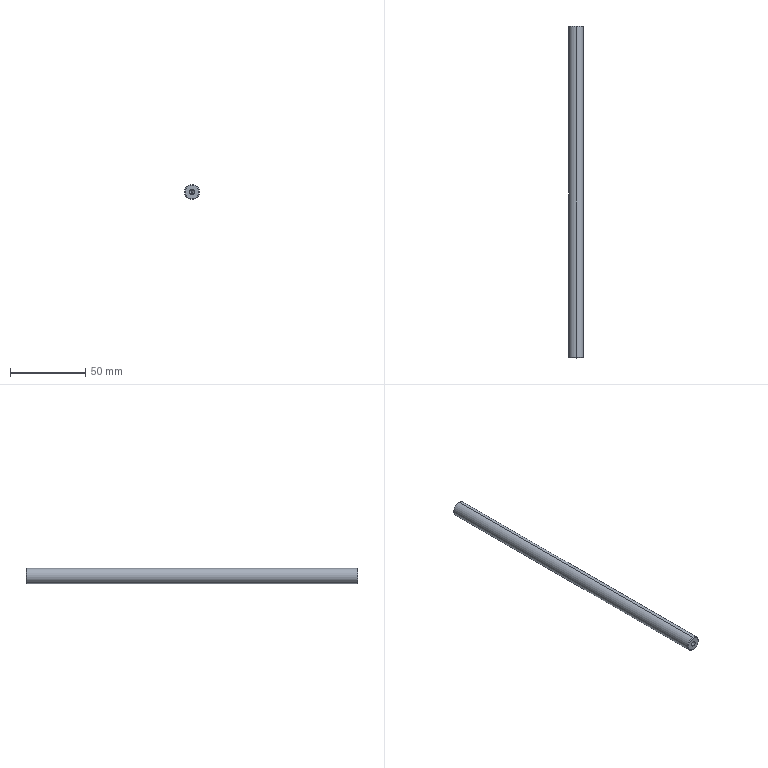Part | SolidWorks | features HoleWzd 2, Chamfer 1, Extrusion 1 | 1 solid | 16 faces | box 10 x 220 x 10 mm | volume 17093 mm3 | cone 8 | cylinder 6 | plane 2 | commonest cylinder face diameters 3.3 x4 10 x2
STEP:
#1=CARTESIAN_POINT('',(0.,-99.9,1.65));
#2=VERTEX_POINT('',#1);
#3=CARTESIAN_POINT('',(0.,-99.9,-1.65));
#4=VERTEX_POINT('',#3);
#5=CARTESIAN_POINT('',(0.,-99.9,0.));
#6=DIRECTION('',(0.,-1.,0.));
#7=DIRECTION('',(0.,0.,-1.));
#8=AXIS2_PLACEMENT_3D('',#5,#6,#7);
#9=CIRCLE('',#8,1.65);
#10=EDGE_CURVE('',#2,#4,#9,.T.);
#11=ORIENTED_EDGE('',*,*,#10,.F.);
#12=CARTESIAN_POINT('',(0.,-110.,1.65));
#13=VERTEX_POINT('',#12);
#14=CARTESIAN_POINT('',(0.,-110.,1.65));
#15=DIRECTION('',(0.,-1.,0.));
#16=VECTOR('',#15,1000.);
#17=LINE('',#14,#16);
#18=EDGE_CURVE('',#2,#13,#17,.T.);
#19=ORIENTED_EDGE('',*,*,#18,.T.);
#20=CARTESIAN_POINT('',(0.,-110.,-1.65));
#21=VERTEX_POINT('',#20);
#22=CARTESIAN_POINT('',(0.,-110.,0.));
#23=DIRECTION('',(0.,-1.,0.));
#24=DIRECTION('',(0.,0.,-1.));
#25=AXIS2_PLACEMENT_3D('',#22,#23,#24);
#26=CIRCLE('',#25,1.65);
#27=EDGE_CURVE('',#13,#21,#26,.T.);
#28=ORIENTED_EDGE('',*,*,#27,.T.);
#29=CARTESIAN_POINT('',(0.,-110.,-1.65));
#30=DIRECTION('',(0.,-1.,0.));
#31=VECTOR('',#30,1000.);
#32=LINE('',#29,#31);
#33=EDGE_CURVE('',#4,#21,#32,.T.);
#34=ORIENTED_EDGE('',*,*,#33,.F.);
#35=EDGE_LOOP('',(#11,#19,#28,#34));
#36=FACE_OUTER_BOUND('',#35,.T.);
#37=CARTESIAN_POINT('',(0.,-110.,0.));
#38=DIRECTION('',(0.,-1.,0.));
#39=DIRECTION('',(0.,0.,-1.));
#40=AXIS2_PLACEMENT_3D('',#37,#38,#39);
#41=CYLINDRICAL_SURFACE('',#40,1.65);
#42=ADVANCED_FACE('',(#36),#41,.F.);
#43=CARTESIAN_POINT('',(0.,-98.909,0.));
#44=VERTEX_POINT('',#43);
#45=CARTESIAN_POINT('',(0.,-99.9,-1.65));
#46=DIRECTION('',(0.,-0.515,-0.8572));
#47=VECTOR('',#46,1000.);
#48=LINE('',#45,#47);
#49=EDGE_CURVE('',#44,#4,#48,.T.);
#50=ORIENTED_EDGE('',*,*,#49,.F.);
#51=CARTESIAN_POINT('',(0.,-99.9,1.65));
#52=DIRECTION('',(0.,-0.515,0.8572));
#53=VECTOR('',#52,1000.);
#54=LINE('',#51,#53);
#55=EDGE_CURVE('',#44,#2,#54,.T.);
#56=ORIENTED_EDGE('',*,*,#55,.T.);
#57=ORIENTED_EDGE('',*,*,#10,.T.);
#58=EDGE_LOOP('',(#50,#56,#57));
#59=FACE_OUTER_BOUND('',#58,.T.);
#60=CARTESIAN_POINT('',(0.,-99.9,0.));
#61=DIRECTION('',(0.,-1.,0.));
#62=DIRECTION('',(0.,0.,-1.));
#63=AXIS2_PLACEMENT_3D('',#60,#61,#62);
#64=CONICAL_SURFACE('',#63,1.65,1.03);
#65=ADVANCED_FACE('',(#59),#64,.F.);
#66=CARTESIAN_POINT('',(0.,99.9,-1.65));
#67=VERTEX_POINT('',#66);
#68=CARTESIAN_POINT('',(0.,99.9,1.65));
#69=VERTEX_POINT('',#68);
#70=CARTESIAN_POINT('',(0.,99.9,0.));
#71=DIRECTION('',(0.,1.,0.));
#72=DIRECTION('',(0.,0.,1.));
#73=AXIS2_PLACEMENT_3D('',#70,#71,#72);
#74=CIRCLE('',#73,1.65);
#75=EDGE_CURVE('',#67,#69,#74,.T.);
#76=ORIENTED_EDGE('',*,*,#75,.F.);
#77=CARTESIAN_POINT('',(0.,110.,-1.65));
#78=VERTEX_POINT('',#77);
#79=CARTESIAN_POINT('',(0.,110.,-1.65));
#80=DIRECTION('',(0.,1.,0.));
#81=VECTOR('',#80,1000.);
#82=LINE('',#79,#81);
#83=EDGE_CURVE('',#67,#78,#82,.T.);
#84=ORIENTED_EDGE('',*,*,#83,.T.);
#85=CARTESIAN_POINT('',(0.,110.,1.65));
#86=VERTEX_POINT('',#85);
#87=CARTESIAN_POINT('',(0.,110.,0.));
#88=DIRECTION('',(0.,1.,0.));
#89=DIRECTION('',(0.,0.,1.));
#90=AXIS2_PLACEMENT_3D('',#87,#88,#89);
#91=CIRCLE('',#90,1.65);
#92=EDGE_CURVE('',#78,#86,#91,.T.);
#93=ORIENTED_EDGE('',*,*,#92,.T.);
#94=CARTESIAN_POINT('',(0.,110.,1.65));
#95=DIRECTION('',(0.,1.,0.));
#96=VECTOR('',#95,1000.);
#97=LINE('',#94,#96);
#98=EDGE_CURVE('',#69,#86,#97,.T.);
#99=ORIENTED_EDGE('',*,*,#98,.F.);
#100=EDGE_LOOP('',(#76,#84,#93,#99));
#101=FACE_OUTER_BOUND('',#100,.T.);
#102=CARTESIAN_POINT('',(0.,110.,0.));
#103=DIRECTION('',(0.,1.,0.));
#104=DIRECTION('',(0.,0.,1.));
#105=AXIS2_PLACEMENT_3D('',#102,#103,#104);
#106=CYLINDRICAL_SURFACE('',#105,1.65);
#107=ADVANCED_FACE('',(#101),#106,.F.);
#108=CARTESIAN_POINT('',(0.,98.909,0.));
#109=VERTEX_POINT('',#108);
#110=CARTESIAN_POINT('',(0.,99.9,1.65));
#111=DIRECTION('',(0.,0.515,0.8572));
#112=VECTOR('',#111,1000.);
#113=LINE('',#110,#112);
#114=EDGE_CURVE('',#109,#69,#113,.T.);
#115=ORIENTED_EDGE('',*,*,#114,.F.);
#116=CARTESIAN_POINT('',(0.,99.9,-1.65));
#117=DIRECTION('',(0.,0.515,-0.8572));
#118=VECTOR('',#117,1000.);
#119=LINE('',#116,#118);
#120=EDGE_CURVE('',#109,#67,#119,.T.);
#121=ORIENTED_EDGE('',*,*,#120,.T.);
#122=ORIENTED_EDGE('',*,*,#75,.T.);
#123=EDGE_LOOP('',(#115,#121,#122));
#124=FACE_OUTER_BOUND('',#123,.T.);
#125=CARTESIAN_POINT('',(0.,99.9,0.));
#126=DIRECTION('',(0.,1.,0.));
#127=DIRECTION('',(0.,0.,1.));
#128=AXIS2_PLACEMENT_3D('',#125,#126,#127);
#129=CONICAL_SURFACE('',#128,1.65,1.03);
#130=ADVANCED_FACE('',(#124),#129,.F.);
#131=CARTESIAN_POINT('',(0.,110.,4.5));
#132=VERTEX_POINT('',#131);
#133=CARTESIAN_POINT('',(0.,110.,-4.5));
#134=VERTEX_POINT('',#133);
#135=CARTESIAN_POINT('',(0.,110.,0.));
#136=DIRECTION('',(0.,1.,0.));
#137=DIRECTION('',(0.,0.,1.));
#138=AXIS2_PLACEMENT_3D('',#135,#136,#137);
#139=CIRCLE('',#138,4.5);
#140=EDGE_CURVE('',#132,#134,#139,.T.);
#141=ORIENTED_EDGE('',*,*,#140,.F.);
#142=CARTESIAN_POINT('',(0.,109.5,5.));
#143=VERTEX_POINT('',#142);
#144=CARTESIAN_POINT('',(0.,110.,4.5));
#145=DIRECTION('',(0.,-0.7071,0.7071));
#146=VECTOR('',#145,1000.);
#147=LINE('',#144,#146);
#148=EDGE_CURVE('',#132,#143,#147,.T.);
#149=ORIENTED_EDGE('',*,*,#148,.T.);
#150=CARTESIAN_POINT('',(0.,109.5,-5.));
#151=VERTEX_POINT('',#150);
#152=CARTESIAN_POINT('',(0.,109.5,0.));
#153=DIRECTION('',(0.,-1.,0.));
#154=DIRECTION('',(0.,0.,1.));
#155=AXIS2_PLACEMENT_3D('',#152,#153,#154);
#156=CIRCLE('',#155,5.);
#157=EDGE_CURVE('',#151,#143,#156,.T.);
#158=ORIENTED_EDGE('',*,*,#157,.F.);
#159=CARTESIAN_POINT('',(0.,110.,-4.5));
#160=DIRECTION('',(0.,-0.7071,-0.7071));
#161=VECTOR('',#160,1000.);
#162=LINE('',#159,#161);
#163=EDGE_CURVE('',#134,#151,#162,.T.);
#164=ORIENTED_EDGE('',*,*,#163,.F.);
#165=EDGE_LOOP('',(#141,#149,#158,#164));
#166=FACE_OUTER_BOUND('',#165,.T.);
#167=CARTESIAN_POINT('',(0.,110.,0.));
#168=DIRECTION('',(0.,-1.,0.));
#169=DIRECTION('',(0.,0.,-1.));
#170=AXIS2_PLACEMENT_3D('',#167,#168,#169);
#171=CONICAL_SURFACE('',#170,4.5,0.7854);
#172=ADVANCED_FACE('',(#166),#171,.T.);
#173=CARTESIAN_POINT('',(0.,-110.,-4.5));
#174=VERTEX_POINT('',#173);
#175=CARTESIAN_POINT('',(0.,-110.,4.5));
#176=VERTEX_POINT('',#175);
#177=CARTESIAN_POINT('',(0.,-110.,0.));
#178=DIRECTION('',(0.,-1.,0.));
#179=DIRECTION('',(0.,0.,1.));
#180=AXIS2_PLACEMENT_3D('',#177,#178,#179);
#181=CIRCLE('',#180,4.5);
#182=EDGE_CURVE('',#174,#176,#181,.T.);
#183=ORIENTED_EDGE('',*,*,#182,.F.);
#184=CARTESIAN_POINT('',(0.,-109.5,-5.));
#185=VERTEX_POINT('',#184);
#186=CARTESIAN_POINT('',(0.,-109.5,-5.));
#187=DIRECTION('',(0.,0.7071,-0.7071));
#188=VECTOR('',#187,1000.);
#189=LINE('',#186,#188);
#190=EDGE_CURVE('',#174,#185,#189,.T.);
#191=ORIENTED_EDGE('',*,*,#190,.T.);
#192=CARTESIAN_POINT('',(0.,-109.5,5.));
#193=VERTEX_POINT('',#192);
#194=CARTESIAN_POINT('',(0.,-109.5,0.));
#195=DIRECTION('',(0.,1.,0.));
#196=DIRECTION('',(0.,0.,1.));
#197=AXIS2_PLACEMENT_3D('',#194,#195,#196);
#198=CIRCLE('',#197,5.);
#199=EDGE_CURVE('',#193,#185,#198,.T.);
#200=ORIENTED_EDGE('',*,*,#199,.F.);
#201=CARTESIAN_POINT('',(0.,-109.5,5.));
#202=DIRECTION('',(0.,0.7071,0.7071));
#203=VECTOR('',#202,1000.);
#204=LINE('',#201,#203);
#205=EDGE_CURVE('',#176,#193,#204,.T.);
#206=ORIENTED_EDGE('',*,*,#205,.F.);
#207=EDGE_LOOP('',(#183,#191,#200,#206));
#208=FACE_OUTER_BOUND('',#207,.T.);
#209=CARTESIAN_POINT('',(0.,-109.5,0.));
#210=DIRECTION('',(0.,1.,0.));
#211=DIRECTION('',(0.,0.,1.));
#212=AXIS2_PLACEMENT_3D('',#209,#210,#211);
#213=CONICAL_SURFACE('',#212,5.,0.7854);
#214=ADVANCED_FACE('',(#208),#213,.T.);
#215=ORIENTED_EDGE('',*,*,#157,.T.);
#216=CARTESIAN_POINT('',(0.,110.,5.));
#217=DIRECTION('',(0.,-1.,0.));
#218=VECTOR('',#217,1000.);
#219=LINE('',#216,#218);
#220=EDGE_CURVE('',#143,#193,#219,.T.);
#221=ORIENTED_EDGE('',*,*,#220,.T.);
#222=ORIENTED_EDGE('',*,*,#199,.T.);
#223=CARTESIAN_POINT('',(0.,110.,-5.));
#224=DIRECTION('',(0.,-1.,0.));
#225=VECTOR('',#224,1000.);
#226=LINE('',#223,#225);
#227=EDGE_CURVE('',#151,#185,#226,.T.);
#228=ORIENTED_EDGE('',*,*,#227,.F.);
#229=EDGE_LOOP('',(#215,#221,#222,#228));
#230=FACE_OUTER_BOUND('',#229,.T.);
#231=CARTESIAN_POINT('',(0.,110.,0.));
#232=DIRECTION('',(0.,-1.,0.));
#233=DIRECTION('',(0.,0.,-1.));
#234=AXIS2_PLACEMENT_3D('',#231,#232,#233);
#235=CYLINDRICAL_SURFACE('',#234,5.);
#236=ADVANCED_FACE('',(#230),#235,.T.);
#237=ORIENTED_EDGE('',*,*,#220,.F.);
#238=CARTESIAN_POINT('',(0.,109.5,0.));
#239=DIRECTION('',(0.,-1.,0.));
#240=DIRECTION('',(0.,0.,1.));
#241=AXIS2_PLACEMENT_3D('',#238,#239,#240);
#242=CIRCLE('',#241,5.);
#243=EDGE_CURVE('',#143,#151,#242,.T.);
#244=ORIENTED_EDGE('',*,*,#243,.T.);
#245=ORIENTED_EDGE('',*,*,#227,.T.);
#246=CARTESIAN_POINT('',(0.,-109.5,0.));
#247=DIRECTION('',(0.,1.,0.));
#248=DIRECTION('',(0.,0.,1.));
#249=AXIS2_PLACEMENT_3D('',#246,#247,#248);
#250=CIRCLE('',#249,5.);
#251=EDGE_CURVE('',#185,#193,#250,.T.);
#252=ORIENTED_EDGE('',*,*,#251,.T.);
#253=EDGE_LOOP('',(#237,#244,#245,#252));
#254=FACE_OUTER_BOUND('',#253,.T.);
#255=CARTESIAN_POINT('',(0.,110.,0.));
#256=DIRECTION('',(0.,-1.,0.));
#257=DIRECTION('',(0.,0.,-1.));
#258=AXIS2_PLACEMENT_3D('',#255,#256,#257);
#259=CYLINDRICAL_SURFACE('',#258,5.);
#260=ADVANCED_FACE('',(#254),#259,.T.);
#261=CARTESIAN_POINT('',(0.,110.,0.));
#262=DIRECTION('',(0.,1.,0.));
#263=DIRECTION('',(0.,0.,1.));
#264=AXIS2_PLACEMENT_3D('',#261,#262,#263);
#265=CIRCLE('',#264,1.65);
#266=EDGE_CURVE('',#86,#78,#265,.T.);
#267=ORIENTED_EDGE('',*,*,#266,.F.);
#268=ORIENTED_EDGE('',*,*,#92,.F.);
#269=EDGE_LOOP('',(#267,#268));
#270=FACE_BOUND('',#269,.T.);
#271=CARTESIAN_POINT('',(0.,110.,0.));
#272=DIRECTION('',(0.,1.,0.));
#273=DIRECTION('',(0.,0.,1.));
#274=AXIS2_PLACEMENT_3D('',#271,#272,#273);
#275=CIRCLE('',#274,4.5);
#276=EDGE_CURVE('',#134,#132,#275,.T.);
#277=ORIENTED_EDGE('',*,*,#276,.T.);
#278=ORIENTED_EDGE('',*,*,#140,.T.);
#279=EDGE_LOOP('',(#277,#278));
#280=FACE_OUTER_BOUND('',#279,.T.);
#281=CARTESIAN_POINT('',(0.,110.,0.));
#282=DIRECTION('',(0.,1.,0.));
#283=DIRECTION('',(0.,0.,1.));
#284=AXIS2_PLACEMENT_3D('',#281,#282,#283);
#285=PLANE('',#284);
#286=ADVANCED_FACE('',(#270,#280),#285,.T.);
#287=CARTESIAN_POINT('',(0.,-110.,0.));
#288=DIRECTION('',(0.,-1.,0.));
#289=DIRECTION('',(0.,0.,-1.));
#290=AXIS2_PLACEMENT_3D('',#287,#288,#289);
#291=CIRCLE('',#290,1.65);
#292=EDGE_CURVE('',#21,#13,#291,.T.);
#293=ORIENTED_EDGE('',*,*,#292,.F.);
#294=ORIENTED_EDGE('',*,*,#27,.F.);
#295=EDGE_LOOP('',(#293,#294));
#296=FACE_BOUND('',#295,.T.);
#297=CARTESIAN_POINT('',(0.,-110.,0.));
#298=DIRECTION('',(0.,-1.,0.));
#299=DIRECTION('',(0.,0.,1.));
#300=AXIS2_PLACEMENT_3D('',#297,#298,#299);
#301=CIRCLE('',#300,4.5);
#302=EDGE_CURVE('',#176,#174,#301,.T.);
#303=ORIENTED_EDGE('',*,*,#302,.T.);
#304=ORIENTED_EDGE('',*,*,#182,.T.);
#305=EDGE_LOOP('',(#303,#304));
#306=FACE_OUTER_BOUND('',#305,.T.);
#307=CARTESIAN_POINT('',(0.,-110.,0.));
#308=DIRECTION('',(0.,1.,0.));
#309=DIRECTION('',(0.,0.,1.));
#310=AXIS2_PLACEMENT_3D('',#307,#308,#309);
#311=PLANE('',#310);
#312=ADVANCED_FACE('',(#296,#306),#311,.F.);
#313=ORIENTED_EDGE('',*,*,#190,.F.);
#314=ORIENTED_EDGE('',*,*,#302,.F.);
#315=ORIENTED_EDGE('',*,*,#205,.T.);
#316=ORIENTED_EDGE('',*,*,#251,.F.);
#317=EDGE_LOOP('',(#313,#314,#315,#316));
#318=FACE_OUTER_BOUND('',#317,.T.);
#319=CARTESIAN_POINT('',(0.,-109.5,0.));
#320=DIRECTION('',(0.,1.,0.));
#321=DIRECTION('',(0.,0.,1.));
#322=AXIS2_PLACEMENT_3D('',#319,#320,#321);
#323=CONICAL_SURFACE('',#322,5.,0.7854);
#324=ADVANCED_FACE('',(#318),#323,.T.);
#325=ORIENTED_EDGE('',*,*,#148,.F.);
#326=ORIENTED_EDGE('',*,*,#276,.F.);
#327=ORIENTED_EDGE('',*,*,#163,.T.);
#328=ORIENTED_EDGE('',*,*,#243,.F.);
#329=EDGE_LOOP('',(#325,#326,#327,#328));
#330=FACE_OUTER_BOUND('',#329,.T.);
#331=CARTESIAN_POINT('',(0.,110.,0.));
#332=DIRECTION('',(0.,-1.,0.));
#333=DIRECTION('',(0.,0.,-1.));
#334=AXIS2_PLACEMENT_3D('',#331,#332,#333);
#335=CONICAL_SURFACE('',#334,4.5,0.7854);
#336=ADVANCED_FACE('',(#330),#335,.T.);
#337=ORIENTED_EDGE('',*,*,#120,.F.);
#338=ORIENTED_EDGE('',*,*,#114,.T.);
#339=CARTESIAN_POINT('',(0.,99.9,0.));
#340=DIRECTION('',(0.,1.,0.));
#341=DIRECTION('',(0.,0.,1.));
#342=AXIS2_PLACEMENT_3D('',#339,#340,#341);
#343=CIRCLE('',#342,1.65);
#344=EDGE_CURVE('',#69,#67,#343,.T.);
#345=ORIENTED_EDGE('',*,*,#344,.T.);
#346=EDGE_LOOP('',(#337,#338,#345));
#347=FACE_OUTER_BOUND('',#346,.T.);
#348=CARTESIAN_POINT('',(0.,99.9,0.));
#349=DIRECTION('',(0.,1.,0.));
#350=DIRECTION('',(0.,0.,1.));
#351=AXIS2_PLACEMENT_3D('',#348,#349,#350);
#352=CONICAL_SURFACE('',#351,1.65,1.03);
#353=ADVANCED_FACE('',(#347),#352,.F.);
#354=ORIENTED_EDGE('',*,*,#83,.F.);
#355=ORIENTED_EDGE('',*,*,#344,.F.);
#356=ORIENTED_EDGE('',*,*,#98,.T.);
#357=ORIENTED_EDGE('',*,*,#266,.T.);
#358=EDGE_LOOP('',(#354,#355,#356,#357));
#359=FACE_OUTER_BOUND('',#358,.T.);
#360=CARTESIAN_POINT('',(0.,110.,0.));
#361=DIRECTION('',(0.,1.,0.));
#362=DIRECTION('',(0.,0.,1.));
#363=AXIS2_PLACEMENT_3D('',#360,#361,#362);
#364=CYLINDRICAL_SURFACE('',#363,1.65);
#365=ADVANCED_FACE('',(#359),#364,.F.);
#366=ORIENTED_EDGE('',*,*,#55,.F.);
#367=ORIENTED_EDGE('',*,*,#49,.T.);
#368=CARTESIAN_POINT('',(0.,-99.9,0.));
#369=DIRECTION('',(0.,-1.,0.));
#370=DIRECTION('',(0.,0.,-1.));
#371=AXIS2_PLACEMENT_3D('',#368,#369,#370);
#372=CIRCLE('',#371,1.65);
#373=EDGE_CURVE('',#4,#2,#372,.T.);
#374=ORIENTED_EDGE('',*,*,#373,.T.);
#375=EDGE_LOOP('',(#366,#367,#374));
#376=FACE_OUTER_BOUND('',#375,.T.);
#377=CARTESIAN_POINT('',(0.,-99.9,0.));
#378=DIRECTION('',(0.,-1.,0.));
#379=DIRECTION('',(0.,0.,-1.));
#380=AXIS2_PLACEMENT_3D('',#377,#378,#379);
#381=CONICAL_SURFACE('',#380,1.65,1.03);
#382=ADVANCED_FACE('',(#376),#381,.F.);
#383=ORIENTED_EDGE('',*,*,#18,.F.);
#384=ORIENTED_EDGE('',*,*,#373,.F.);
#385=ORIENTED_EDGE('',*,*,#33,.T.);
#386=ORIENTED_EDGE('',*,*,#292,.T.);
#387=EDGE_LOOP('',(#383,#384,#385,#386));
#388=FACE_OUTER_BOUND('',#387,.T.);
#389=CARTESIAN_POINT('',(0.,-110.,0.));
#390=DIRECTION('',(0.,-1.,0.));
#391=DIRECTION('',(0.,0.,-1.));
#392=AXIS2_PLACEMENT_3D('',#389,#390,#391);
#393=CYLINDRICAL_SURFACE('',#392,1.65);
#394=ADVANCED_FACE('',(#388),#393,.F.);
#395=CLOSED_SHELL('',(#42,#65,#107,#130,#172,#214,#236,#260,#286,#312,#324,#336,#353,#365,#382,#394));
#396=MANIFOLD_SOLID_BREP('',#395);
#397=CARTESIAN_POINT('',(0.,0.,0.));
#398=DIRECTION('',(0.,0.,1.));
#399=DIRECTION('',(1.,0.,0.));
#400=AXIS2_PLACEMENT_3D('',#397,#398,#399);
#401=(LENGTH_UNIT()NAMED_UNIT(*)SI_UNIT(.MILLI.,.METRE.));
#402=UNCERTAINTY_MEASURE_WITH_UNIT(LENGTH_MEASURE(0.00001),#401,'','');
#403=(NAMED_UNIT(*)PLANE_ANGLE_UNIT()SI_UNIT($,.RADIAN.));
#404=(NAMED_UNIT(*)SI_UNIT($,.STERADIAN.)SOLID_ANGLE_UNIT());
#405=(GEOMETRIC_REPRESENTATION_CONTEXT(3)GLOBAL_UNCERTAINTY_ASSIGNED_CONTEXT((#402))GLOBAL_UNIT_ASSIGNED_CONTEXT((#401,#403,#404))REPRESENTATION_CONTEXT('',''));
#406=ADVANCED_BREP_SHAPE_REPRESENTATION('',(#396,#400),#405);